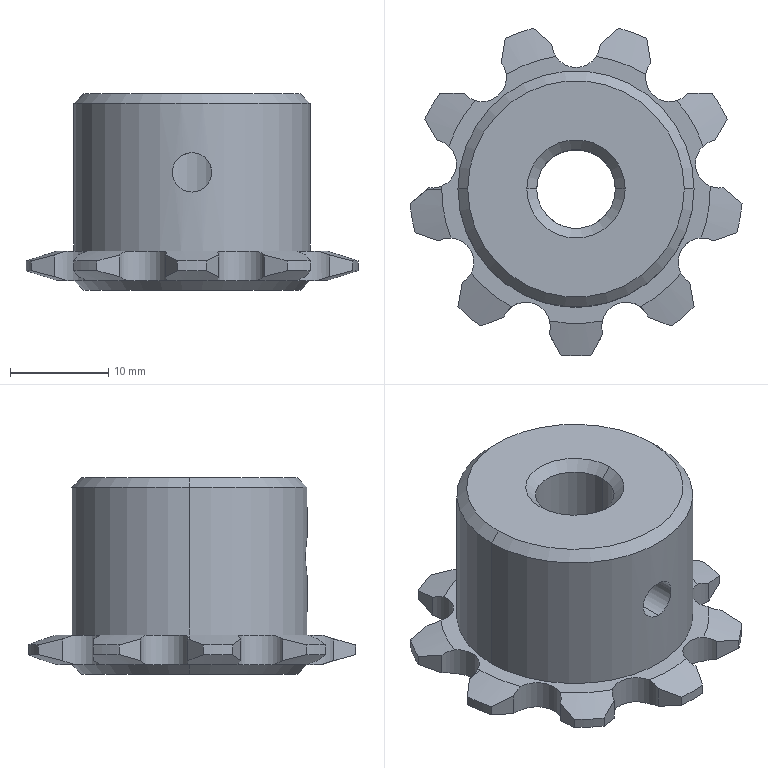Part | STEP file | Sprocket | 1 solid | 83 faces | box 33.749 x 33.304 x 20 mm | volume 8415 mm3 | cone 29 | cylinder 28 | plane 26 | commonest cylinder face diameters 4.913 x13 33.87 x9 4 x2 8 x2 24 x2